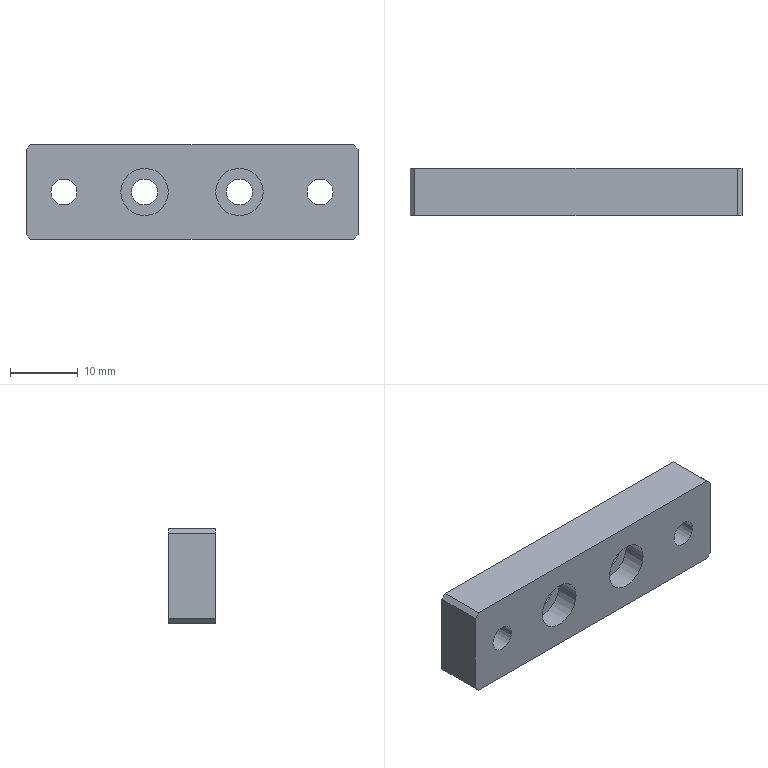Part | SolidWorks | features SplitBody 1 | 1 solid | 30 faces | box 49 x 7 x 14 mm | volume 4093 mm3 | cylinder 16 | plane 14 | commonest cylinder face diameters 3.85 x8 7 x8
STEP:
#1=CARTESIAN_POINT('',(446.475,106.359,-264.316));
#2=VERTEX_POINT('',#1);
#3=CARTESIAN_POINT('',(439.475,106.359,-264.316));
#4=VERTEX_POINT('',#3);
#5=CARTESIAN_POINT('',(442.975,106.359,-264.316));
#6=DIRECTION('',(0.,1.,0.));
#7=DIRECTION('',(-1.,0.,0.));
#8=AXIS2_PLACEMENT_3D('',#5,#6,#7);
#9=CIRCLE('',#8,3.5);
#10=EDGE_CURVE('',#2,#4,#9,.T.);
#11=ORIENTED_EDGE('',*,*,#10,.F.);
#12=CARTESIAN_POINT('',(446.475,109.859,-264.316));
#13=VERTEX_POINT('',#12);
#14=CARTESIAN_POINT('',(446.475,109.859,-264.316));
#15=DIRECTION('',(0.,1.,0.));
#16=VECTOR('',#15,1000.);
#17=LINE('',#14,#16);
#18=EDGE_CURVE('',#2,#13,#17,.T.);
#19=ORIENTED_EDGE('',*,*,#18,.T.);
#20=CARTESIAN_POINT('',(439.475,109.859,-264.316));
#21=VERTEX_POINT('',#20);
#22=CARTESIAN_POINT('',(442.975,109.859,-264.316));
#23=DIRECTION('',(0.,1.,0.));
#24=DIRECTION('',(-1.,0.,0.));
#25=AXIS2_PLACEMENT_3D('',#22,#23,#24);
#26=CIRCLE('',#25,3.5);
#27=EDGE_CURVE('',#13,#21,#26,.T.);
#28=ORIENTED_EDGE('',*,*,#27,.T.);
#29=CARTESIAN_POINT('',(439.475,109.859,-264.316));
#30=DIRECTION('',(0.,1.,0.));
#31=VECTOR('',#30,1000.);
#32=LINE('',#29,#31);
#33=EDGE_CURVE('',#4,#21,#32,.T.);
#34=ORIENTED_EDGE('',*,*,#33,.F.);
#35=EDGE_LOOP('',(#11,#19,#28,#34));
#36=FACE_OUTER_BOUND('',#35,.T.);
#37=CARTESIAN_POINT('',(442.975,109.859,-264.316));
#38=DIRECTION('',(0.,1.,0.));
#39=DIRECTION('',(-1.,0.,0.));
#40=AXIS2_PLACEMENT_3D('',#37,#38,#39);
#41=CYLINDRICAL_SURFACE('',#40,3.5);
#42=ADVANCED_FACE('',(#36),#41,.F.);
#43=CARTESIAN_POINT('',(444.9,102.859,-264.316));
#44=VERTEX_POINT('',#43);
#45=CARTESIAN_POINT('',(441.05,102.859,-264.316));
#46=VERTEX_POINT('',#45);
#47=CARTESIAN_POINT('',(442.975,102.859,-264.316));
#48=DIRECTION('',(0.,1.,0.));
#49=DIRECTION('',(-1.,0.,0.));
#50=AXIS2_PLACEMENT_3D('',#47,#48,#49);
#51=CIRCLE('',#50,1.925);
#52=EDGE_CURVE('',#44,#46,#51,.T.);
#53=ORIENTED_EDGE('',*,*,#52,.F.);
#54=CARTESIAN_POINT('',(444.9,106.359,-264.316));
#55=VERTEX_POINT('',#54);
#56=CARTESIAN_POINT('',(444.9,109.859,-264.316));
#57=DIRECTION('',(0.,1.,0.));
#58=VECTOR('',#57,1000.);
#59=LINE('',#56,#58);
#60=EDGE_CURVE('',#44,#55,#59,.T.);
#61=ORIENTED_EDGE('',*,*,#60,.T.);
#62=CARTESIAN_POINT('',(441.05,106.359,-264.316));
#63=VERTEX_POINT('',#62);
#64=CARTESIAN_POINT('',(442.975,106.359,-264.316));
#65=DIRECTION('',(0.,1.,0.));
#66=DIRECTION('',(-1.,0.,0.));
#67=AXIS2_PLACEMENT_3D('',#64,#65,#66);
#68=CIRCLE('',#67,1.925);
#69=EDGE_CURVE('',#55,#63,#68,.T.);
#70=ORIENTED_EDGE('',*,*,#69,.T.);
#71=CARTESIAN_POINT('',(441.05,109.859,-264.316));
#72=DIRECTION('',(0.,1.,0.));
#73=VECTOR('',#72,1000.);
#74=LINE('',#71,#73);
#75=EDGE_CURVE('',#46,#63,#74,.T.);
#76=ORIENTED_EDGE('',*,*,#75,.F.);
#77=EDGE_LOOP('',(#53,#61,#70,#76));
#78=FACE_OUTER_BOUND('',#77,.T.);
#79=CARTESIAN_POINT('',(442.975,109.859,-264.316));
#80=DIRECTION('',(0.,1.,0.));
#81=DIRECTION('',(-1.,0.,0.));
#82=AXIS2_PLACEMENT_3D('',#79,#80,#81);
#83=CYLINDRICAL_SURFACE('',#82,1.925);
#84=ADVANCED_FACE('',(#78),#83,.F.);
#85=CARTESIAN_POINT('',(408.675,106.359,-264.316));
#86=VERTEX_POINT('',#85);
#87=CARTESIAN_POINT('',(401.675,106.359,-264.316));
#88=VERTEX_POINT('',#87);
#89=CARTESIAN_POINT('',(405.175,106.359,-264.316));
#90=DIRECTION('',(0.,1.,0.));
#91=DIRECTION('',(-1.,0.,0.));
#92=AXIS2_PLACEMENT_3D('',#89,#90,#91);
#93=CIRCLE('',#92,3.5);
#94=EDGE_CURVE('',#86,#88,#93,.T.);
#95=ORIENTED_EDGE('',*,*,#94,.F.);
#96=CARTESIAN_POINT('',(408.675,109.859,-264.316));
#97=VERTEX_POINT('',#96);
#98=CARTESIAN_POINT('',(408.675,109.859,-264.316));
#99=DIRECTION('',(0.,1.,0.));
#100=VECTOR('',#99,1000.);
#101=LINE('',#98,#100);
#102=EDGE_CURVE('',#86,#97,#101,.T.);
#103=ORIENTED_EDGE('',*,*,#102,.T.);
#104=CARTESIAN_POINT('',(401.675,109.859,-264.316));
#105=VERTEX_POINT('',#104);
#106=CARTESIAN_POINT('',(405.175,109.859,-264.316));
#107=DIRECTION('',(0.,1.,0.));
#108=DIRECTION('',(-1.,0.,0.));
#109=AXIS2_PLACEMENT_3D('',#106,#107,#108);
#110=CIRCLE('',#109,3.5);
#111=EDGE_CURVE('',#97,#105,#110,.T.);
#112=ORIENTED_EDGE('',*,*,#111,.T.);
#113=CARTESIAN_POINT('',(401.675,109.859,-264.316));
#114=DIRECTION('',(0.,1.,0.));
#115=VECTOR('',#114,1000.);
#116=LINE('',#113,#115);
#117=EDGE_CURVE('',#88,#105,#116,.T.);
#118=ORIENTED_EDGE('',*,*,#117,.F.);
#119=EDGE_LOOP('',(#95,#103,#112,#118));
#120=FACE_OUTER_BOUND('',#119,.T.);
#121=CARTESIAN_POINT('',(405.175,109.859,-264.316));
#122=DIRECTION('',(0.,1.,0.));
#123=DIRECTION('',(-1.,0.,0.));
#124=AXIS2_PLACEMENT_3D('',#121,#122,#123);
#125=CYLINDRICAL_SURFACE('',#124,3.5);
#126=ADVANCED_FACE('',(#120),#125,.F.);
#127=CARTESIAN_POINT('',(407.1,102.859,-264.316));
#128=VERTEX_POINT('',#127);
#129=CARTESIAN_POINT('',(403.25,102.859,-264.316));
#130=VERTEX_POINT('',#129);
#131=CARTESIAN_POINT('',(405.175,102.859,-264.316));
#132=DIRECTION('',(0.,1.,0.));
#133=DIRECTION('',(-1.,0.,0.));
#134=AXIS2_PLACEMENT_3D('',#131,#132,#133);
#135=CIRCLE('',#134,1.925);
#136=EDGE_CURVE('',#128,#130,#135,.T.);
#137=ORIENTED_EDGE('',*,*,#136,.F.);
#138=CARTESIAN_POINT('',(407.1,106.359,-264.316));
#139=VERTEX_POINT('',#138);
#140=CARTESIAN_POINT('',(407.1,109.859,-264.316));
#141=DIRECTION('',(0.,1.,0.));
#142=VECTOR('',#141,1000.);
#143=LINE('',#140,#142);
#144=EDGE_CURVE('',#128,#139,#143,.T.);
#145=ORIENTED_EDGE('',*,*,#144,.T.);
#146=CARTESIAN_POINT('',(403.25,106.359,-264.316));
#147=VERTEX_POINT('',#146);
#148=CARTESIAN_POINT('',(405.175,106.359,-264.316));
#149=DIRECTION('',(0.,1.,0.));
#150=DIRECTION('',(-1.,0.,0.));
#151=AXIS2_PLACEMENT_3D('',#148,#149,#150);
#152=CIRCLE('',#151,1.925);
#153=EDGE_CURVE('',#139,#147,#152,.T.);
#154=ORIENTED_EDGE('',*,*,#153,.T.);
#155=CARTESIAN_POINT('',(403.25,109.859,-264.316));
#156=DIRECTION('',(0.,1.,0.));
#157=VECTOR('',#156,1000.);
#158=LINE('',#155,#157);
#159=EDGE_CURVE('',#130,#147,#158,.T.);
#160=ORIENTED_EDGE('',*,*,#159,.F.);
#161=EDGE_LOOP('',(#137,#145,#154,#160));
#162=FACE_OUTER_BOUND('',#161,.T.);
#163=CARTESIAN_POINT('',(405.175,109.859,-264.316));
#164=DIRECTION('',(0.,1.,0.));
#165=DIRECTION('',(-1.,0.,0.));
#166=AXIS2_PLACEMENT_3D('',#163,#164,#165);
#167=CYLINDRICAL_SURFACE('',#166,1.925);
#168=ADVANCED_FACE('',(#162),#167,.F.);
#169=CARTESIAN_POINT('',(413.575,106.359,-264.316));
#170=VERTEX_POINT('',#169);
#171=CARTESIAN_POINT('',(420.575,106.359,-264.316));
#172=VERTEX_POINT('',#171);
#173=CARTESIAN_POINT('',(417.075,106.359,-264.316));
#174=DIRECTION('',(0.,-1.,0.));
#175=DIRECTION('',(1.,0.,0.));
#176=AXIS2_PLACEMENT_3D('',#173,#174,#175);
#177=CIRCLE('',#176,3.5);
#178=EDGE_CURVE('',#170,#172,#177,.T.);
#179=ORIENTED_EDGE('',*,*,#178,.F.);
#180=CARTESIAN_POINT('',(413.575,102.859,-264.316));
#181=VERTEX_POINT('',#180);
#182=CARTESIAN_POINT('',(413.575,102.859,-264.316));
#183=DIRECTION('',(0.,-1.,0.));
#184=VECTOR('',#183,1000.);
#185=LINE('',#182,#184);
#186=EDGE_CURVE('',#170,#181,#185,.T.);
#187=ORIENTED_EDGE('',*,*,#186,.T.);
#188=CARTESIAN_POINT('',(420.575,102.859,-264.316));
#189=VERTEX_POINT('',#188);
#190=CARTESIAN_POINT('',(417.075,102.859,-264.316));
#191=DIRECTION('',(0.,-1.,0.));
#192=DIRECTION('',(1.,0.,0.));
#193=AXIS2_PLACEMENT_3D('',#190,#191,#192);
#194=CIRCLE('',#193,3.5);
#195=EDGE_CURVE('',#181,#189,#194,.T.);
#196=ORIENTED_EDGE('',*,*,#195,.T.);
#197=CARTESIAN_POINT('',(420.575,102.859,-264.316));
#198=DIRECTION('',(0.,-1.,0.));
#199=VECTOR('',#198,1000.);
#200=LINE('',#197,#199);
#201=EDGE_CURVE('',#172,#189,#200,.T.);
#202=ORIENTED_EDGE('',*,*,#201,.F.);
#203=EDGE_LOOP('',(#179,#187,#196,#202));
#204=FACE_OUTER_BOUND('',#203,.T.);
#205=CARTESIAN_POINT('',(417.075,102.859,-264.316));
#206=DIRECTION('',(0.,-1.,0.));
#207=DIRECTION('',(1.,0.,0.));
#208=AXIS2_PLACEMENT_3D('',#205,#206,#207);
#209=CYLINDRICAL_SURFACE('',#208,3.5);
#210=ADVANCED_FACE('',(#204),#209,.F.);
#211=CARTESIAN_POINT('',(415.15,109.859,-264.316));
#212=VERTEX_POINT('',#211);
#213=CARTESIAN_POINT('',(419.,109.859,-264.316));
#214=VERTEX_POINT('',#213);
#215=CARTESIAN_POINT('',(417.075,109.859,-264.316));
#216=DIRECTION('',(0.,-1.,0.));
#217=DIRECTION('',(1.,0.,0.));
#218=AXIS2_PLACEMENT_3D('',#215,#216,#217);
#219=CIRCLE('',#218,1.925);
#220=EDGE_CURVE('',#212,#214,#219,.T.);
#221=ORIENTED_EDGE('',*,*,#220,.F.);
#222=CARTESIAN_POINT('',(415.15,106.359,-264.316));
#223=VERTEX_POINT('',#222);
#224=CARTESIAN_POINT('',(415.15,102.859,-264.316));
#225=DIRECTION('',(0.,-1.,0.));
#226=VECTOR('',#225,1000.);
#227=LINE('',#224,#226);
#228=EDGE_CURVE('',#212,#223,#227,.T.);
#229=ORIENTED_EDGE('',*,*,#228,.T.);
#230=CARTESIAN_POINT('',(419.,106.359,-264.316));
#231=VERTEX_POINT('',#230);
#232=CARTESIAN_POINT('',(417.075,106.359,-264.316));
#233=DIRECTION('',(0.,-1.,0.));
#234=DIRECTION('',(1.,0.,0.));
#235=AXIS2_PLACEMENT_3D('',#232,#233,#234);
#236=CIRCLE('',#235,1.925);
#237=EDGE_CURVE('',#223,#231,#236,.T.);
#238=ORIENTED_EDGE('',*,*,#237,.T.);
#239=CARTESIAN_POINT('',(419.,102.859,-264.316));
#240=DIRECTION('',(0.,-1.,0.));
#241=VECTOR('',#240,1000.);
#242=LINE('',#239,#241);
#243=EDGE_CURVE('',#214,#231,#242,.T.);
#244=ORIENTED_EDGE('',*,*,#243,.F.);
#245=EDGE_LOOP('',(#221,#229,#238,#244));
#246=FACE_OUTER_BOUND('',#245,.T.);
#247=CARTESIAN_POINT('',(417.075,102.859,-264.316));
#248=DIRECTION('',(0.,-1.,0.));
#249=DIRECTION('',(1.,0.,0.));
#250=AXIS2_PLACEMENT_3D('',#247,#248,#249);
#251=CYLINDRICAL_SURFACE('',#250,1.925);
#252=ADVANCED_FACE('',(#246),#251,.F.);
#253=CARTESIAN_POINT('',(427.575,106.359,-264.316));
#254=VERTEX_POINT('',#253);
#255=CARTESIAN_POINT('',(434.575,106.359,-264.316));
#256=VERTEX_POINT('',#255);
#257=CARTESIAN_POINT('',(431.075,106.359,-264.316));
#258=DIRECTION('',(0.,-1.,0.));
#259=DIRECTION('',(1.,0.,0.));
#260=AXIS2_PLACEMENT_3D('',#257,#258,#259);
#261=CIRCLE('',#260,3.5);
#262=EDGE_CURVE('',#254,#256,#261,.T.);
#263=ORIENTED_EDGE('',*,*,#262,.F.);
#264=CARTESIAN_POINT('',(427.575,102.859,-264.316));
#265=VERTEX_POINT('',#264);
#266=CARTESIAN_POINT('',(427.575,102.859,-264.316));
#267=DIRECTION('',(0.,-1.,0.));
#268=VECTOR('',#267,1000.);
#269=LINE('',#266,#268);
#270=EDGE_CURVE('',#254,#265,#269,.T.);
#271=ORIENTED_EDGE('',*,*,#270,.T.);
#272=CARTESIAN_POINT('',(434.575,102.859,-264.316));
#273=VERTEX_POINT('',#272);
#274=CARTESIAN_POINT('',(431.075,102.859,-264.316));
#275=DIRECTION('',(0.,-1.,0.));
#276=DIRECTION('',(1.,0.,0.));
#277=AXIS2_PLACEMENT_3D('',#274,#275,#276);
#278=CIRCLE('',#277,3.5);
#279=EDGE_CURVE('',#265,#273,#278,.T.);
#280=ORIENTED_EDGE('',*,*,#279,.T.);
#281=CARTESIAN_POINT('',(434.575,102.859,-264.316));
#282=DIRECTION('',(0.,-1.,0.));
#283=VECTOR('',#282,1000.);
#284=LINE('',#281,#283);
#285=EDGE_CURVE('',#256,#273,#284,.T.);
#286=ORIENTED_EDGE('',*,*,#285,.F.);
#287=EDGE_LOOP('',(#263,#271,#280,#286));
#288=FACE_OUTER_BOUND('',#287,.T.);
#289=CARTESIAN_POINT('',(431.075,102.859,-264.316));
#290=DIRECTION('',(0.,-1.,0.));
#291=DIRECTION('',(1.,0.,0.));
#292=AXIS2_PLACEMENT_3D('',#289,#290,#291);
#293=CYLINDRICAL_SURFACE('',#292,3.5);
#294=ADVANCED_FACE('',(#288),#293,.F.);
#295=CARTESIAN_POINT('',(429.15,109.859,-264.316));
#296=VERTEX_POINT('',#295);
#297=CARTESIAN_POINT('',(433.,109.859,-264.316));
#298=VERTEX_POINT('',#297);
#299=CARTESIAN_POINT('',(431.075,109.859,-264.316));
#300=DIRECTION('',(0.,-1.,0.));
#301=DIRECTION('',(1.,0.,0.));
#302=AXIS2_PLACEMENT_3D('',#299,#300,#301);
#303=CIRCLE('',#302,1.925);
#304=EDGE_CURVE('',#296,#298,#303,.T.);
#305=ORIENTED_EDGE('',*,*,#304,.F.);
#306=CARTESIAN_POINT('',(429.15,106.359,-264.316));
#307=VERTEX_POINT('',#306);
#308=CARTESIAN_POINT('',(429.15,102.859,-264.316));
#309=DIRECTION('',(0.,-1.,0.));
#310=VECTOR('',#309,1000.);
#311=LINE('',#308,#310);
#312=EDGE_CURVE('',#296,#307,#311,.T.);
#313=ORIENTED_EDGE('',*,*,#312,.T.);
#314=CARTESIAN_POINT('',(433.,106.359,-264.316));
#315=VERTEX_POINT('',#314);
#316=CARTESIAN_POINT('',(431.075,106.359,-264.316));
#317=DIRECTION('',(0.,-1.,0.));
#318=DIRECTION('',(1.,0.,0.));
#319=AXIS2_PLACEMENT_3D('',#316,#317,#318);
#320=CIRCLE('',#319,1.925);
#321=EDGE_CURVE('',#307,#315,#320,.T.);
#322=ORIENTED_EDGE('',*,*,#321,.T.);
#323=CARTESIAN_POINT('',(433.,102.859,-264.316));
#324=DIRECTION('',(0.,-1.,0.));
#325=VECTOR('',#324,1000.);
#326=LINE('',#323,#325);
#327=EDGE_CURVE('',#298,#315,#326,.T.);
#328=ORIENTED_EDGE('',*,*,#327,.F.);
#329=EDGE_LOOP('',(#305,#313,#322,#328));
#330=FACE_OUTER_BOUND('',#329,.T.);
#331=CARTESIAN_POINT('',(431.075,102.859,-264.316));
#332=DIRECTION('',(0.,-1.,0.));
#333=DIRECTION('',(1.,0.,0.));
#334=AXIS2_PLACEMENT_3D('',#331,#332,#333);
#335=CYLINDRICAL_SURFACE('',#334,1.925);
#336=ADVANCED_FACE('',(#330),#335,.F.);
#337=CARTESIAN_POINT('',(448.575,102.859,-258.016));
#338=VERTEX_POINT('',#337);
#339=CARTESIAN_POINT('',(448.575,102.859,-270.616));
#340=VERTEX_POINT('',#339);
#341=CARTESIAN_POINT('',(448.575,102.859,-271.316));
#342=DIRECTION('',(0.,0.,-1.));
#343=VECTOR('',#342,1000.);
#344=LINE('',#341,#343);
#345=EDGE_CURVE('',#338,#340,#344,.T.);
#346=ORIENTED_EDGE('',*,*,#345,.T.);
#347=CARTESIAN_POINT('',(448.575,109.859,-270.616));
#348=VERTEX_POINT('',#347);
#349=CARTESIAN_POINT('',(448.575,109.859,-270.616));
#350=DIRECTION('',(0.,1.,0.));
#351=VECTOR('',#350,1000.);
#352=LINE('',#349,#351);
#353=EDGE_CURVE('',#340,#348,#352,.T.);
#354=ORIENTED_EDGE('',*,*,#353,.T.);
#355=CARTESIAN_POINT('',(448.575,109.859,-258.016));
#356=VERTEX_POINT('',#355);
#357=CARTESIAN_POINT('',(448.575,109.859,-271.316));
#358=DIRECTION('',(0.,0.,-1.));
#359=VECTOR('',#358,1000.);
#360=LINE('',#357,#359);
#361=EDGE_CURVE('',#356,#348,#360,.T.);
#362=ORIENTED_EDGE('',*,*,#361,.F.);
#363=CARTESIAN_POINT('',(448.575,109.859,-258.016));
#364=DIRECTION('',(0.,-1.,0.));
#365=VECTOR('',#364,1000.);
#366=LINE('',#363,#365);
#367=EDGE_CURVE('',#356,#338,#366,.T.);
#368=ORIENTED_EDGE('',*,*,#367,.T.);
#369=EDGE_LOOP('',(#346,#354,#362,#368));
#370=FACE_OUTER_BOUND('',#369,.T.);
#371=CARTESIAN_POINT('',(448.575,109.859,-271.316));
#372=DIRECTION('',(-1.,0.,0.));
#373=DIRECTION('',(0.,-1.,0.));
#374=AXIS2_PLACEMENT_3D('',#371,#372,#373);
#375=PLANE('',#374);
#376=ADVANCED_FACE('',(#370),#375,.F.);
#377=CARTESIAN_POINT('',(447.875,102.859,-271.316));
#378=VERTEX_POINT('',#377);
#379=CARTESIAN_POINT('',(400.275,102.859,-271.316));
#380=VERTEX_POINT('',#379);
#381=CARTESIAN_POINT('',(448.575,102.859,-271.316));
#382=DIRECTION('',(-1.,0.,0.));
#383=VECTOR('',#382,1000.);
#384=LINE('',#381,#383);
#385=EDGE_CURVE('',#378,#380,#384,.T.);
#386=ORIENTED_EDGE('',*,*,#385,.T.);
#387=CARTESIAN_POINT('',(400.275,109.859,-271.316));
#388=VERTEX_POINT('',#387);
#389=CARTESIAN_POINT('',(400.275,109.859,-271.316));
#390=DIRECTION('',(0.,1.,0.));
#391=VECTOR('',#390,1000.);
#392=LINE('',#389,#391);
#393=EDGE_CURVE('',#380,#388,#392,.T.);
#394=ORIENTED_EDGE('',*,*,#393,.T.);
#395=CARTESIAN_POINT('',(447.875,109.859,-271.316));
#396=VERTEX_POINT('',#395);
#397=CARTESIAN_POINT('',(448.575,109.859,-271.316));
#398=DIRECTION('',(-1.,0.,0.));
#399=VECTOR('',#398,1000.);
#400=LINE('',#397,#399);
#401=EDGE_CURVE('',#396,#388,#400,.T.);
#402=ORIENTED_EDGE('',*,*,#401,.F.);
#403=CARTESIAN_POINT('',(447.875,109.859,-271.316));
#404=DIRECTION('',(0.,-1.,0.));
#405=VECTOR('',#404,1000.);
#406=LINE('',#403,#405);
#407=EDGE_CURVE('',#396,#378,#406,.T.);
#408=ORIENTED_EDGE('',*,*,#407,.T.);
#409=EDGE_LOOP('',(#386,#394,#402,#408));
#410=FACE_OUTER_BOUND('',#409,.T.);
#411=CARTESIAN_POINT('',(448.575,109.859,-271.316));
#412=DIRECTION('',(0.,0.,1.));
#413=DIRECTION('',(0.,1.,0.));
#414=AXIS2_PLACEMENT_3D('',#411,#412,#413);
#415=PLANE('',#414);
#416=ADVANCED_FACE('',(#410),#415,.F.);
#417=CARTESIAN_POINT('',(399.575,109.859,-270.616));
#418=VERTEX_POINT('',#417);
#419=CARTESIAN_POINT('',(399.575,109.859,-258.016));
#420=VERTEX_POINT('',#419);
#421=CARTESIAN_POINT('',(399.575,109.859,-271.316));
#422=DIRECTION('',(0.,0.,1.));
#423=VECTOR('',#422,1000.);
#424=LINE('',#421,#423);
#425=EDGE_CURVE('',#418,#420,#424,.T.);
#426=ORIENTED_EDGE('',*,*,#425,.F.);
#427=CARTESIAN_POINT('',(399.575,102.859,-270.616));
#428=VERTEX_POINT('',#427);
#429=CARTESIAN_POINT('',(399.575,109.859,-270.616));
#430=DIRECTION('',(0.,-1.,0.));
#431=VECTOR('',#430,1000.);
#432=LINE('',#429,#431);
#433=EDGE_CURVE('',#418,#428,#432,.T.);
#434=ORIENTED_EDGE('',*,*,#433,.T.);
#435=CARTESIAN_POINT('',(399.575,102.859,-258.016));
#436=VERTEX_POINT('',#435);
#437=CARTESIAN_POINT('',(399.575,102.859,-271.316));
#438=DIRECTION('',(0.,0.,1.));
#439=VECTOR('',#438,1000.);
#440=LINE('',#437,#439);
#441=EDGE_CURVE('',#428,#436,#440,.T.);
#442=ORIENTED_EDGE('',*,*,#441,.T.);
#443=CARTESIAN_POINT('',(399.575,109.859,-258.016));
#444=DIRECTION('',(0.,1.,0.));
#445=VECTOR('',#444,1000.);
#446=LINE('',#443,#445);
#447=EDGE_CURVE('',#436,#420,#446,.T.);
#448=ORIENTED_EDGE('',*,*,#447,.T.);
#449=EDGE_LOOP('',(#426,#434,#442,#448));
#450=FACE_OUTER_BOUND('',#449,.T.);
#451=CARTESIAN_POINT('',(399.575,109.859,-271.316));
#452=DIRECTION('',(1.,0.,0.));
#453=DIRECTION('',(0.,1.,0.));
#454=AXIS2_PLACEMENT_3D('',#451,#452,#453);
#455=PLANE('',#454);
#456=ADVANCED_FACE('',(#450),#455,.F.);
#457=CARTESIAN_POINT('',(400.275,109.859,-257.316));
#458=VERTEX_POINT('',#457);
#459=CARTESIAN_POINT('',(447.875,109.859,-257.316));
#460=VERTEX_POINT('',#459);
#461=CARTESIAN_POINT('',(448.575,109.859,-257.316));
#462=DIRECTION('',(1.,0.,0.));
#463=VECTOR('',#462,1000.);
#464=LINE('',#461,#463);
#465=EDGE_CURVE('',#458,#460,#464,.T.);
#466=ORIENTED_EDGE('',*,*,#465,.F.);
#467=CARTESIAN_POINT('',(400.275,102.859,-257.316));
#468=VERTEX_POINT('',#467);
#469=CARTESIAN_POINT('',(400.275,109.859,-257.316));
#470=DIRECTION('',(0.,-1.,0.));
#471=VECTOR('',#470,1000.);
#472=LINE('',#469,#471);
#473=EDGE_CURVE('',#458,#468,#472,.T.);
#474=ORIENTED_EDGE('',*,*,#473,.T.);
#475=CARTESIAN_POINT('',(447.875,102.859,-257.316));
#476=VERTEX_POINT('',#475);
#477=CARTESIAN_POINT('',(448.575,102.859,-257.316));
#478=DIRECTION('',(1.,0.,0.));
#479=VECTOR('',#478,1000.);
#480=LINE('',#477,#479);
#481=EDGE_CURVE('',#468,#476,#480,.T.);
#482=ORIENTED_EDGE('',*,*,#481,.T.);
#483=CARTESIAN_POINT('',(447.875,109.859,-257.316));
#484=DIRECTION('',(0.,1.,0.));
#485=VECTOR('',#484,1000.);
#486=LINE('',#483,#485);
#487=EDGE_CURVE('',#476,#460,#486,.T.);
#488=ORIENTED_EDGE('',*,*,#487,.T.);
#489=EDGE_LOOP('',(#466,#474,#482,#488));
#490=FACE_OUTER_BOUND('',#489,.T.);
#491=CARTESIAN_POINT('',(448.575,109.859,-257.316));
#492=DIRECTION('',(0.,0.,-1.));
#493=DIRECTION('',(0.,-1.,0.));
#494=AXIS2_PLACEMENT_3D('',#491,#492,#493);
#495=PLANE('',#494);
#496=ADVANCED_FACE('',(#490),#495,.F.);
#497=CARTESIAN_POINT('',(442.975,109.859,-264.316));
#498=DIRECTION('',(0.,1.,0.));
#499=DIRECTION('',(-1.,0.,0.));
#500=AXIS2_PLACEMENT_3D('',#497,#498,#499);
#501=CIRCLE('',#500,3.5);
#502=EDGE_CURVE('',#21,#13,#501,.T.);
#503=ORIENTED_EDGE('',*,*,#502,.F.);
#504=ORIENTED_EDGE('',*,*,#27,.F.);
#505=EDGE_LOOP('',(#503,#504));
#506=FACE_BOUND('',#505,.T.);
#507=CARTESIAN_POINT('',(405.175,109.859,-264.316));
#508=DIRECTION('',(0.,1.,0.));
#509=DIRECTION('',(-1.,0.,0.));
#510=AXIS2_PLACEMENT_3D('',#507,#508,#509);
#511=CIRCLE('',#510,3.5);
#512=EDGE_CURVE('',#105,#97,#511,.T.);
#513=ORIENTED_EDGE('',*,*,#512,.F.);
#514=ORIENTED_EDGE('',*,*,#111,.F.);
#515=EDGE_LOOP('',(#513,#514));
#516=FACE_BOUND('',#515,.T.);
#517=CARTESIAN_POINT('',(417.075,109.859,-264.316));
#518=DIRECTION('',(0.,-1.,0.));
#519=DIRECTION('',(1.,0.,0.));
#520=AXIS2_PLACEMENT_3D('',#517,#518,#519);
#521=CIRCLE('',#520,1.925);
#522=EDGE_CURVE('',#214,#212,#521,.T.);
#523=ORIENTED_EDGE('',*,*,#522,.T.);
#524=ORIENTED_EDGE('',*,*,#220,.T.);
#525=EDGE_LOOP('',(#523,#524));
#526=FACE_BOUND('',#525,.T.);
#527=CARTESIAN_POINT('',(431.075,109.859,-264.316));
#528=DIRECTION('',(0.,-1.,0.));
#529=DIRECTION('',(1.,0.,0.));
#530=AXIS2_PLACEMENT_3D('',#527,#528,#529);
#531=CIRCLE('',#530,1.925);
#532=EDGE_CURVE('',#298,#296,#531,.T.);
#533=ORIENTED_EDGE('',*,*,#532,.T.);
#534=ORIENTED_EDGE('',*,*,#304,.T.);
#535=EDGE_LOOP('',(#533,#534));
#536=FACE_BOUND('',#535,.T.);
#537=ORIENTED_EDGE('',*,*,#401,.T.);
#538=CARTESIAN_POINT('',(399.575,109.859,-270.616));
#539=DIRECTION('',(-0.7071,0.,0.7071));
#540=VECTOR('',#539,1000.);
#541=LINE('',#538,#540);
#542=EDGE_CURVE('',#388,#418,#541,.T.);
#543=ORIENTED_EDGE('',*,*,#542,.T.);
#544=ORIENTED_EDGE('',*,*,#425,.T.);
#545=CARTESIAN_POINT('',(400.275,109.859,-257.316));
#546=DIRECTION('',(0.7071,0.,0.7071));
#547=VECTOR('',#546,1000.);
#548=LINE('',#545,#547);
#549=EDGE_CURVE('',#420,#458,#548,.T.);
#550=ORIENTED_EDGE('',*,*,#549,.T.);
#551=ORIENTED_EDGE('',*,*,#465,.T.);
#552=CARTESIAN_POINT('',(448.575,109.859,-258.016));
#553=DIRECTION('',(0.7071,0.,-0.7071));
#554=VECTOR('',#553,1000.);
#555=LINE('',#552,#554);
#556=EDGE_CURVE('',#460,#356,#555,.T.);
#557=ORIENTED_EDGE('',*,*,#556,.T.);
#558=ORIENTED_EDGE('',*,*,#361,.T.);
#559=CARTESIAN_POINT('',(447.875,109.859,-271.316));
#560=DIRECTION('',(-0.7071,0.,-0.7071));
#561=VECTOR('',#560,1000.);
#562=LINE('',#559,#561);
#563=EDGE_CURVE('',#348,#396,#562,.T.);
#564=ORIENTED_EDGE('',*,*,#563,.T.);
#565=EDGE_LOOP('',(#537,#543,#544,#550,#551,#557,#558,#564));
#566=FACE_OUTER_BOUND('',#565,.T.);
#567=CARTESIAN_POINT('',(448.575,109.859,-257.316));
#568=DIRECTION('',(0.,-1.,0.));
#569=DIRECTION('',(1.,0.,0.));
#570=AXIS2_PLACEMENT_3D('',#567,#568,#569);
#571=PLANE('',#570);
#572=ADVANCED_FACE('',(#506,#516,#526,#536,#566),#571,.F.);
#573=CARTESIAN_POINT('',(442.975,102.859,-264.316));
#574=DIRECTION('',(0.,1.,0.));
#575=DIRECTION('',(-1.,0.,0.));
#576=AXIS2_PLACEMENT_3D('',#573,#574,#575);
#577=CIRCLE('',#576,1.925);
#578=EDGE_CURVE('',#46,#44,#577,.T.);
#579=ORIENTED_EDGE('',*,*,#578,.T.);
#580=ORIENTED_EDGE('',*,*,#52,.T.);
#581=EDGE_LOOP('',(#579,#580));
#582=FACE_BOUND('',#581,.T.);
#583=CARTESIAN_POINT('',(405.175,102.859,-264.316));
#584=DIRECTION('',(0.,1.,0.));
#585=DIRECTION('',(-1.,0.,0.));
#586=AXIS2_PLACEMENT_3D('',#583,#584,#585);
#587=CIRCLE('',#586,1.925);
#588=EDGE_CURVE('',#130,#128,#587,.T.);
#589=ORIENTED_EDGE('',*,*,#588,.T.);
#590=ORIENTED_EDGE('',*,*,#136,.T.);
#591=EDGE_LOOP('',(#589,#590));
#592=FACE_BOUND('',#591,.T.);
#593=CARTESIAN_POINT('',(417.075,102.859,-264.316));
#594=DIRECTION('',(0.,-1.,0.));
#595=DIRECTION('',(1.,0.,0.));
#596=AXIS2_PLACEMENT_3D('',#593,#594,#595);
#597=CIRCLE('',#596,3.5);
#598=EDGE_CURVE('',#189,#181,#597,.T.);
#599=ORIENTED_EDGE('',*,*,#598,.F.);
#600=ORIENTED_EDGE('',*,*,#195,.F.);
#601=EDGE_LOOP('',(#599,#600));
#602=FACE_BOUND('',#601,.T.);
#603=CARTESIAN_POINT('',(431.075,102.859,-264.316));
#604=DIRECTION('',(0.,-1.,0.));
#605=DIRECTION('',(1.,0.,0.));
#606=AXIS2_PLACEMENT_3D('',#603,#604,#605);
#607=CIRCLE('',#606,3.5);
#608=EDGE_CURVE('',#273,#265,#607,.T.);
#609=ORIENTED_EDGE('',*,*,#608,.F.);
#610=ORIENTED_EDGE('',*,*,#279,.F.);
#611=EDGE_LOOP('',(#609,#610));
#612=FACE_BOUND('',#611,.T.);
#613=ORIENTED_EDGE('',*,*,#441,.F.);
#614=CARTESIAN_POINT('',(417.425,102.859,-288.466));
#615=DIRECTION('',(0.7071,0.,-0.7071));
#616=VECTOR('',#615,1000.);
#617=LINE('',#614,#616);
#618=EDGE_CURVE('',#428,#380,#617,.T.);
#619=ORIENTED_EDGE('',*,*,#618,.T.);
#620=ORIENTED_EDGE('',*,*,#385,.F.);
#621=CARTESIAN_POINT('',(455.225,102.859,-263.966));
#622=DIRECTION('',(0.7071,0.,0.7071));
#623=VECTOR('',#622,1000.);
#624=LINE('',#621,#623);
#625=EDGE_CURVE('',#378,#340,#624,.T.);
#626=ORIENTED_EDGE('',*,*,#625,.T.);
#627=ORIENTED_EDGE('',*,*,#345,.F.);
#628=CARTESIAN_POINT('',(448.225,102.859,-257.666));
#629=DIRECTION('',(-0.7071,0.,0.7071));
#630=VECTOR('',#629,1000.);
#631=LINE('',#628,#630);
#632=EDGE_CURVE('',#338,#476,#631,.T.);
#633=ORIENTED_EDGE('',*,*,#632,.T.);
#634=ORIENTED_EDGE('',*,*,#481,.F.);
#635=CARTESIAN_POINT('',(424.425,102.859,-233.166));
#636=DIRECTION('',(-0.7071,0.,-0.7071));
#637=VECTOR('',#636,1000.);
#638=LINE('',#635,#637);
#639=EDGE_CURVE('',#468,#436,#638,.T.);
#640=ORIENTED_EDGE('',*,*,#639,.T.);
#641=EDGE_LOOP('',(#613,#619,#620,#626,#627,#633,#634,#640));
#642=FACE_OUTER_BOUND('',#641,.T.);
#643=CARTESIAN_POINT('',(448.575,102.859,-257.316));
#644=DIRECTION('',(0.,-1.,0.));
#645=DIRECTION('',(1.,0.,0.));
#646=AXIS2_PLACEMENT_3D('',#643,#644,#645);
#647=PLANE('',#646);
#648=ADVANCED_FACE('',(#582,#592,#602,#612,#642),#647,.T.);
#649=ORIENTED_EDGE('',*,*,#312,.F.);
#650=ORIENTED_EDGE('',*,*,#532,.F.);
#651=ORIENTED_EDGE('',*,*,#327,.T.);
#652=CARTESIAN_POINT('',(431.075,106.359,-264.316));
#653=DIRECTION('',(0.,-1.,0.));
#654=DIRECTION('',(1.,0.,0.));
#655=AXIS2_PLACEMENT_3D('',#652,#653,#654);
#656=CIRCLE('',#655,1.925);
#657=EDGE_CURVE('',#315,#307,#656,.T.);
#658=ORIENTED_EDGE('',*,*,#657,.T.);
#659=EDGE_LOOP('',(#649,#650,#651,#658));
#660=FACE_OUTER_BOUND('',#659,.T.);
#661=CARTESIAN_POINT('',(431.075,102.859,-264.316));
#662=DIRECTION('',(0.,-1.,0.));
#663=DIRECTION('',(1.,0.,0.));
#664=AXIS2_PLACEMENT_3D('',#661,#662,#663);
#665=CYLINDRICAL_SURFACE('',#664,1.925);
#666=ADVANCED_FACE('',(#660),#665,.F.);
#667=ORIENTED_EDGE('',*,*,#657,.F.);
#668=ORIENTED_EDGE('',*,*,#321,.F.);
#669=EDGE_LOOP('',(#667,#668));
#670=FACE_BOUND('',#669,.T.);
#671=CARTESIAN_POINT('',(431.075,106.359,-264.316));
#672=DIRECTION('',(0.,-1.,0.));
#673=DIRECTION('',(1.,0.,0.));
#674=AXIS2_PLACEMENT_3D('',#671,#672,#673);
#675=CIRCLE('',#674,3.5);
#676=EDGE_CURVE('',#256,#254,#675,.T.);
#677=ORIENTED_EDGE('',*,*,#676,.T.);
#678=ORIENTED_EDGE('',*,*,#262,.T.);
#679=EDGE_LOOP('',(#677,#678));
#680=FACE_OUTER_BOUND('',#679,.T.);
#681=CARTESIAN_POINT('',(429.15,106.359,-264.316));
#682=DIRECTION('',(0.,1.,0.));
#683=DIRECTION('',(-1.,0.,0.));
#684=AXIS2_PLACEMENT_3D('',#681,#682,#683);
#685=PLANE('',#684);
#686=ADVANCED_FACE('',(#670,#680),#685,.F.);
#687=ORIENTED_EDGE('',*,*,#270,.F.);
#688=ORIENTED_EDGE('',*,*,#676,.F.);
#689=ORIENTED_EDGE('',*,*,#285,.T.);
#690=ORIENTED_EDGE('',*,*,#608,.T.);
#691=EDGE_LOOP('',(#687,#688,#689,#690));
#692=FACE_OUTER_BOUND('',#691,.T.);
#693=CARTESIAN_POINT('',(431.075,102.859,-264.316));
#694=DIRECTION('',(0.,-1.,0.));
#695=DIRECTION('',(1.,0.,0.));
#696=AXIS2_PLACEMENT_3D('',#693,#694,#695);
#697=CYLINDRICAL_SURFACE('',#696,3.5);
#698=ADVANCED_FACE('',(#692),#697,.F.);
#699=ORIENTED_EDGE('',*,*,#228,.F.);
#700=ORIENTED_EDGE('',*,*,#522,.F.);
#701=ORIENTED_EDGE('',*,*,#243,.T.);
#702=CARTESIAN_POINT('',(417.075,106.359,-264.316));
#703=DIRECTION('',(0.,-1.,0.));
#704=DIRECTION('',(1.,0.,0.));
#705=AXIS2_PLACEMENT_3D('',#702,#703,#704);
#706=CIRCLE('',#705,1.925);
#707=EDGE_CURVE('',#231,#223,#706,.T.);
#708=ORIENTED_EDGE('',*,*,#707,.T.);
#709=EDGE_LOOP('',(#699,#700,#701,#708));
#710=FACE_OUTER_BOUND('',#709,.T.);
#711=CARTESIAN_POINT('',(417.075,102.859,-264.316));
#712=DIRECTION('',(0.,-1.,0.));
#713=DIRECTION('',(1.,0.,0.));
#714=AXIS2_PLACEMENT_3D('',#711,#712,#713);
#715=CYLINDRICAL_SURFACE('',#714,1.925);
#716=ADVANCED_FACE('',(#710),#715,.F.);
#717=ORIENTED_EDGE('',*,*,#707,.F.);
#718=ORIENTED_EDGE('',*,*,#237,.F.);
#719=EDGE_LOOP('',(#717,#718));
#720=FACE_BOUND('',#719,.T.);
#721=CARTESIAN_POINT('',(417.075,106.359,-264.316));
#722=DIRECTION('',(0.,-1.,0.));
#723=DIRECTION('',(1.,0.,0.));
#724=AXIS2_PLACEMENT_3D('',#721,#722,#723);
#725=CIRCLE('',#724,3.5);
#726=EDGE_CURVE('',#172,#170,#725,.T.);
#727=ORIENTED_EDGE('',*,*,#726,.T.);
#728=ORIENTED_EDGE('',*,*,#178,.T.);
#729=EDGE_LOOP('',(#727,#728));
#730=FACE_OUTER_BOUND('',#729,.T.);
#731=CARTESIAN_POINT('',(415.15,106.359,-264.316));
#732=DIRECTION('',(0.,1.,0.));
#733=DIRECTION('',(-1.,0.,0.));
#734=AXIS2_PLACEMENT_3D('',#731,#732,#733);
#735=PLANE('',#734);
#736=ADVANCED_FACE('',(#720,#730),#735,.F.);
#737=ORIENTED_EDGE('',*,*,#186,.F.);
#738=ORIENTED_EDGE('',*,*,#726,.F.);
#739=ORIENTED_EDGE('',*,*,#201,.T.);
#740=ORIENTED_EDGE('',*,*,#598,.T.);
#741=EDGE_LOOP('',(#737,#738,#739,#740));
#742=FACE_OUTER_BOUND('',#741,.T.);
#743=CARTESIAN_POINT('',(417.075,102.859,-264.316));
#744=DIRECTION('',(0.,-1.,0.));
#745=DIRECTION('',(1.,0.,0.));
#746=AXIS2_PLACEMENT_3D('',#743,#744,#745);
#747=CYLINDRICAL_SURFACE('',#746,3.5);
#748=ADVANCED_FACE('',(#742),#747,.F.);
#749=ORIENTED_EDGE('',*,*,#144,.F.);
#750=ORIENTED_EDGE('',*,*,#588,.F.);
#751=ORIENTED_EDGE('',*,*,#159,.T.);
#752=CARTESIAN_POINT('',(405.175,106.359,-264.316));
#753=DIRECTION('',(0.,1.,0.));
#754=DIRECTION('',(-1.,0.,0.));
#755=AXIS2_PLACEMENT_3D('',#752,#753,#754);
#756=CIRCLE('',#755,1.925);
#757=EDGE_CURVE('',#147,#139,#756,.T.);
#758=ORIENTED_EDGE('',*,*,#757,.T.);
#759=EDGE_LOOP('',(#749,#750,#751,#758));
#760=FACE_OUTER_BOUND('',#759,.T.);
#761=CARTESIAN_POINT('',(405.175,109.859,-264.316));
#762=DIRECTION('',(0.,1.,0.));
#763=DIRECTION('',(-1.,0.,0.));
#764=AXIS2_PLACEMENT_3D('',#761,#762,#763);
#765=CYLINDRICAL_SURFACE('',#764,1.925);
#766=ADVANCED_FACE('',(#760),#765,.F.);
#767=ORIENTED_EDGE('',*,*,#757,.F.);
#768=ORIENTED_EDGE('',*,*,#153,.F.);
#769=EDGE_LOOP('',(#767,#768));
#770=FACE_BOUND('',#769,.T.);
#771=CARTESIAN_POINT('',(405.175,106.359,-264.316));
#772=DIRECTION('',(0.,1.,0.));
#773=DIRECTION('',(-1.,0.,0.));
#774=AXIS2_PLACEMENT_3D('',#771,#772,#773);
#775=CIRCLE('',#774,3.5);
#776=EDGE_CURVE('',#88,#86,#775,.T.);
#777=ORIENTED_EDGE('',*,*,#776,.T.);
#778=ORIENTED_EDGE('',*,*,#94,.T.);
#779=EDGE_LOOP('',(#777,#778));
#780=FACE_OUTER_BOUND('',#779,.T.);
#781=CARTESIAN_POINT('',(403.25,106.359,-264.316));
#782=DIRECTION('',(0.,-1.,0.));
#783=DIRECTION('',(1.,0.,0.));
#784=AXIS2_PLACEMENT_3D('',#781,#782,#783);
#785=PLANE('',#784);
#786=ADVANCED_FACE('',(#770,#780),#785,.F.);
#787=ORIENTED_EDGE('',*,*,#102,.F.);
#788=ORIENTED_EDGE('',*,*,#776,.F.);
#789=ORIENTED_EDGE('',*,*,#117,.T.);
#790=ORIENTED_EDGE('',*,*,#512,.T.);
#791=EDGE_LOOP('',(#787,#788,#789,#790));
#792=FACE_OUTER_BOUND('',#791,.T.);
#793=CARTESIAN_POINT('',(405.175,109.859,-264.316));
#794=DIRECTION('',(0.,1.,0.));
#795=DIRECTION('',(-1.,0.,0.));
#796=AXIS2_PLACEMENT_3D('',#793,#794,#795);
#797=CYLINDRICAL_SURFACE('',#796,3.5);
#798=ADVANCED_FACE('',(#792),#797,.F.);
#799=ORIENTED_EDGE('',*,*,#60,.F.);
#800=ORIENTED_EDGE('',*,*,#578,.F.);
#801=ORIENTED_EDGE('',*,*,#75,.T.);
#802=CARTESIAN_POINT('',(442.975,106.359,-264.316));
#803=DIRECTION('',(0.,1.,0.));
#804=DIRECTION('',(-1.,0.,0.));
#805=AXIS2_PLACEMENT_3D('',#802,#803,#804);
#806=CIRCLE('',#805,1.925);
#807=EDGE_CURVE('',#63,#55,#806,.T.);
#808=ORIENTED_EDGE('',*,*,#807,.T.);
#809=EDGE_LOOP('',(#799,#800,#801,#808));
#810=FACE_OUTER_BOUND('',#809,.T.);
#811=CARTESIAN_POINT('',(442.975,109.859,-264.316));
#812=DIRECTION('',(0.,1.,0.));
#813=DIRECTION('',(-1.,0.,0.));
#814=AXIS2_PLACEMENT_3D('',#811,#812,#813);
#815=CYLINDRICAL_SURFACE('',#814,1.925);
#816=ADVANCED_FACE('',(#810),#815,.F.);
#817=ORIENTED_EDGE('',*,*,#807,.F.);
#818=ORIENTED_EDGE('',*,*,#69,.F.);
#819=EDGE_LOOP('',(#817,#818));
#820=FACE_BOUND('',#819,.T.);
#821=CARTESIAN_POINT('',(442.975,106.359,-264.316));
#822=DIRECTION('',(0.,1.,0.));
#823=DIRECTION('',(-1.,0.,0.));
#824=AXIS2_PLACEMENT_3D('',#821,#822,#823);
#825=CIRCLE('',#824,3.5);
#826=EDGE_CURVE('',#4,#2,#825,.T.);
#827=ORIENTED_EDGE('',*,*,#826,.T.);
#828=ORIENTED_EDGE('',*,*,#10,.T.);
#829=EDGE_LOOP('',(#827,#828));
#830=FACE_OUTER_BOUND('',#829,.T.);
#831=CARTESIAN_POINT('',(441.05,106.359,-264.316));
#832=DIRECTION('',(0.,-1.,0.));
#833=DIRECTION('',(1.,0.,0.));
#834=AXIS2_PLACEMENT_3D('',#831,#832,#833);
#835=PLANE('',#834);
#836=ADVANCED_FACE('',(#820,#830),#835,.F.);
#837=ORIENTED_EDGE('',*,*,#18,.F.);
#838=ORIENTED_EDGE('',*,*,#826,.F.);
#839=ORIENTED_EDGE('',*,*,#33,.T.);
#840=ORIENTED_EDGE('',*,*,#502,.T.);
#841=EDGE_LOOP('',(#837,#838,#839,#840));
#842=FACE_OUTER_BOUND('',#841,.T.);
#843=CARTESIAN_POINT('',(442.975,109.859,-264.316));
#844=DIRECTION('',(0.,1.,0.));
#845=DIRECTION('',(-1.,0.,0.));
#846=AXIS2_PLACEMENT_3D('',#843,#844,#845);
#847=CYLINDRICAL_SURFACE('',#846,3.5);
#848=ADVANCED_FACE('',(#842),#847,.F.);
#849=ORIENTED_EDGE('',*,*,#542,.F.);
#850=ORIENTED_EDGE('',*,*,#393,.F.);
#851=ORIENTED_EDGE('',*,*,#618,.F.);
#852=ORIENTED_EDGE('',*,*,#433,.F.);
#853=EDGE_LOOP('',(#849,#850,#851,#852));
#854=FACE_OUTER_BOUND('',#853,.T.);
#855=CARTESIAN_POINT('',(399.575,109.859,-270.616));
#856=DIRECTION('',(0.7071,0.,0.7071));
#857=DIRECTION('',(0.7071,0.,-0.7071));
#858=AXIS2_PLACEMENT_3D('',#855,#856,#857);
#859=PLANE('',#858);
#860=ADVANCED_FACE('',(#854),#859,.F.);
#861=ORIENTED_EDGE('',*,*,#563,.F.);
#862=ORIENTED_EDGE('',*,*,#353,.F.);
#863=ORIENTED_EDGE('',*,*,#625,.F.);
#864=ORIENTED_EDGE('',*,*,#407,.F.);
#865=EDGE_LOOP('',(#861,#862,#863,#864));
#866=FACE_OUTER_BOUND('',#865,.T.);
#867=CARTESIAN_POINT('',(447.875,109.859,-271.316));
#868=DIRECTION('',(-0.7071,0.,0.7071));
#869=DIRECTION('',(0.7071,0.,0.7071));
#870=AXIS2_PLACEMENT_3D('',#867,#868,#869);
#871=PLANE('',#870);
#872=ADVANCED_FACE('',(#866),#871,.F.);
#873=ORIENTED_EDGE('',*,*,#549,.F.);
#874=ORIENTED_EDGE('',*,*,#447,.F.);
#875=ORIENTED_EDGE('',*,*,#639,.F.);
#876=ORIENTED_EDGE('',*,*,#473,.F.);
#877=EDGE_LOOP('',(#873,#874,#875,#876));
#878=FACE_OUTER_BOUND('',#877,.T.);
#879=CARTESIAN_POINT('',(400.275,109.859,-257.316));
#880=DIRECTION('',(0.7071,0.,-0.7071));
#881=DIRECTION('',(-0.7071,0.,-0.7071));
#882=AXIS2_PLACEMENT_3D('',#879,#880,#881);
#883=PLANE('',#882);
#884=ADVANCED_FACE('',(#878),#883,.F.);
#885=ORIENTED_EDGE('',*,*,#556,.F.);
#886=ORIENTED_EDGE('',*,*,#487,.F.);
#887=ORIENTED_EDGE('',*,*,#632,.F.);
#888=ORIENTED_EDGE('',*,*,#367,.F.);
#889=EDGE_LOOP('',(#885,#886,#887,#888));
#890=FACE_OUTER_BOUND('',#889,.T.);
#891=CARTESIAN_POINT('',(448.575,109.859,-258.016));
#892=DIRECTION('',(-0.7071,0.,-0.7071));
#893=DIRECTION('',(-0.7071,0.,0.7071));
#894=AXIS2_PLACEMENT_3D('',#891,#892,#893);
#895=PLANE('',#894);
#896=ADVANCED_FACE('',(#890),#895,.F.);
#897=CLOSED_SHELL('',(#42,#84,#126,#168,#210,#252,#294,#336,#376,#416,#456,#496,#572,#648,#666,#686,#698,#716,#736,#748,#766,#786,#798,#816,#836,#848,#860,#872,#884,#896));
#898=MANIFOLD_SOLID_BREP('',#897);
#899=CARTESIAN_POINT('',(0.,0.,0.));
#900=DIRECTION('',(0.,0.,1.));
#901=DIRECTION('',(1.,0.,0.));
#902=AXIS2_PLACEMENT_3D('',#899,#900,#901);
#903=(LENGTH_UNIT()NAMED_UNIT(*)SI_UNIT(.MILLI.,.METRE.));
#904=UNCERTAINTY_MEASURE_WITH_UNIT(LENGTH_MEASURE(0.00001),#903,'','');
#905=(NAMED_UNIT(*)PLANE_ANGLE_UNIT()SI_UNIT($,.RADIAN.));
#906=(NAMED_UNIT(*)SI_UNIT($,.STERADIAN.)SOLID_ANGLE_UNIT());
#907=(GEOMETRIC_REPRESENTATION_CONTEXT(3)GLOBAL_UNCERTAINTY_ASSIGNED_CONTEXT((#904))GLOBAL_UNIT_ASSIGNED_CONTEXT((#903,#905,#906))REPRESENTATION_CONTEXT('',''));
#908=ADVANCED_BREP_SHAPE_REPRESENTATION('',(#898,#902),#907);